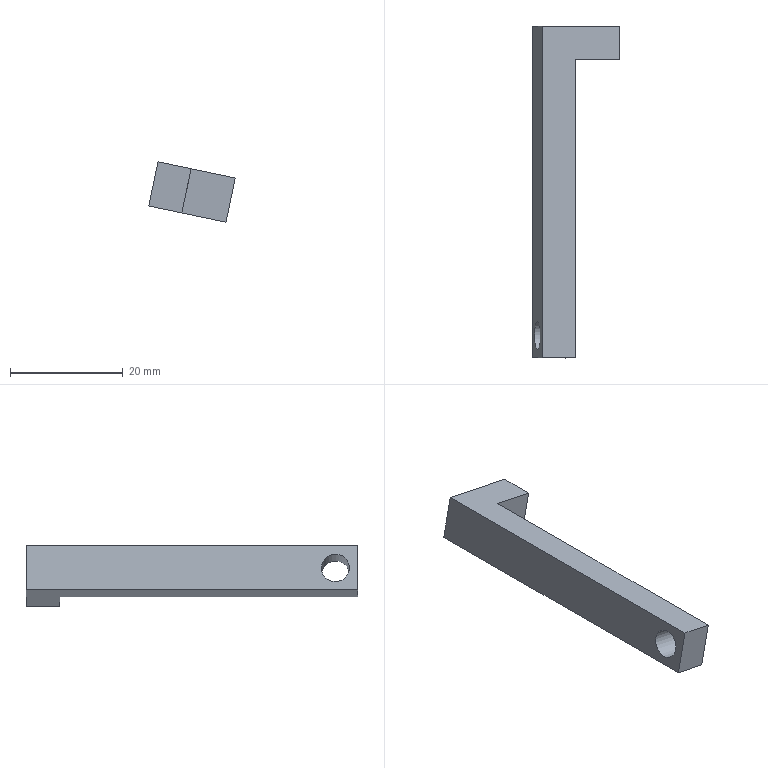Part | STEP file | SN10_006_003_GUIA | 1 solid | 9 faces | box 15.346 x 59 x 10.708 mm | volume 3098 mm3 | plane 8 | cylinder 1 | commonest cylinder face diameters 5 x1
STEP:
#1=CARTESIAN_POINT('',(0.,0.,0.));
#2=DIRECTION('',(0.,0.,1.));
#3=DIRECTION('',(1.,0.,0.));
#4=AXIS2_PLACEMENT_3D('',#1,#2,#3);
#5=CARTESIAN_POINT('',(355.51,-536.049,335.898));
#6=VERTEX_POINT('',#5);
#7=CARTESIAN_POINT('',(355.059,-534.85,333.75));
#8=DIRECTION('',(-0.9786,0.,0.2056));
#9=DIRECTION('',(0.2056,0.,0.9786));
#10=AXIS2_PLACEMENT_3D('',#7,#8,#9);
#11=CIRCLE('',#10,2.5);
#12=CARTESIAN_POINT('',(355.157,-534.85,333.73));
#13=DIRECTION('',(0.9786,0.,-0.2056));
#14=DIRECTION('',(0.1805,-0.4794,0.8588));
#15=AXIS2_PLACEMENT_3D('',#12,#13,#14);
#16=CYLINDRICAL_SURFACE('',#15,2.5);
#17=CARTESIAN_POINT('',(12.066,-0.1));
#18=DIRECTION('',(-1.,0.));
#19=VECTOR('',#18,1.);
#20=LINE('',#17,#19);
#21=(GEOMETRIC_REPRESENTATION_CONTEXT(2)PARAMETRIC_REPRESENTATION_CONTEXT()REPRESENTATION_CONTEXT('',''));
#22=DEFINITIONAL_REPRESENTATION('',(#20),#21);
#23=PCURVE('',#16,#22);
#24=CARTESIAN_POINT('',(355.059,-479.85,333.75));
#25=DIRECTION('',(-0.9786,0.,0.2056));
#26=DIRECTION('',(0.2056,0.,0.9786));
#27=AXIS2_PLACEMENT_3D('',#24,#25,#26);
#28=PLANE('',#27);
#29=CARTESIAN_POINT('',(0.,-55.));
#30=DIRECTION('',(1.,0.));
#31=AXIS2_PLACEMENT_2D('',#29,#30);
#32=CIRCLE('',#31,2.5);
#33=(GEOMETRIC_REPRESENTATION_CONTEXT(2)PARAMETRIC_REPRESENTATION_CONTEXT()REPRESENTATION_CONTEXT('',''));
#34=DEFINITIONAL_REPRESENTATION('',(#32),#33);
#35=PCURVE('',#28,#34);
#36=SURFACE_CURVE('',#11,(#23,#35),.PCURVE_S1.);
#37=EDGE_CURVE('',#6,#6,#36,.T.);
#38=ORIENTED_EDGE('',*,*,#37,.F.);
#39=CARTESIAN_POINT('',(361.382,-536.049,334.664));
#40=VERTEX_POINT('',#39);
#41=CARTESIAN_POINT('',(355.51,-536.049,335.898));
#42=CARTESIAN_POINT('',(361.382,-536.049,334.664));
#43=B_SPLINE_CURVE_WITH_KNOTS('',1,(#41,#42),.UNSPECIFIED.,.F.,.F.,(2,2),(-0.1,5.9),.PIECEWISE_BEZIER_KNOTS.);
#44=CARTESIAN_POINT('',(6.283,0.));
#45=DIRECTION('',(0.,1.));
#46=VECTOR('',#45,1.);
#47=LINE('',#44,#46);
#48=(GEOMETRIC_REPRESENTATION_CONTEXT(2)PARAMETRIC_REPRESENTATION_CONTEXT()REPRESENTATION_CONTEXT('',''));
#49=DEFINITIONAL_REPRESENTATION('',(#47),#48);
#50=PCURVE('',#16,#49);
#51=CARTESIAN_POINT('',(0.,0.));
#52=DIRECTION('',(0.,1.));
#53=VECTOR('',#52,1.);
#54=LINE('',#51,#53);
#55=(GEOMETRIC_REPRESENTATION_CONTEXT(2)PARAMETRIC_REPRESENTATION_CONTEXT()REPRESENTATION_CONTEXT('',''));
#56=DEFINITIONAL_REPRESENTATION('',(#54),#55);
#57=PCURVE('',#16,#56);
#58=SEAM_CURVE('',#43,(#50,#57),.PCURVE_S1.);
#59=EDGE_CURVE('',#6,#40,#58,.T.);
#60=ORIENTED_EDGE('',*,*,#59,.T.);
#61=CARTESIAN_POINT('',(360.931,-534.85,332.517));
#62=DIRECTION('',(0.9786,0.,-0.2056));
#63=DIRECTION('',(0.2056,0.,0.9786));
#64=AXIS2_PLACEMENT_3D('',#61,#62,#63);
#65=CIRCLE('',#64,2.5);
#66=CARTESIAN_POINT('',(-0.5,5.9));
#67=DIRECTION('',(1.,0.));
#68=VECTOR('',#67,1.);
#69=LINE('',#66,#68);
#70=(GEOMETRIC_REPRESENTATION_CONTEXT(2)PARAMETRIC_REPRESENTATION_CONTEXT()REPRESENTATION_CONTEXT('',''));
#71=DEFINITIONAL_REPRESENTATION('',(#69),#70);
#72=PCURVE('',#16,#71);
#73=CARTESIAN_POINT('',(360.931,-538.85,332.517));
#74=DIRECTION('',(0.9786,0.,-0.2056));
#75=DIRECTION('',(-0.2056,0.,-0.9786));
#76=AXIS2_PLACEMENT_3D('',#73,#74,#75);
#77=PLANE('',#76);
#78=CARTESIAN_POINT('',(0.,4.));
#79=DIRECTION('',(-1.,0.));
#80=AXIS2_PLACEMENT_2D('',#78,#79);
#81=CIRCLE('',#80,2.5);
#82=(GEOMETRIC_REPRESENTATION_CONTEXT(2)PARAMETRIC_REPRESENTATION_CONTEXT()REPRESENTATION_CONTEXT('',''));
#83=DEFINITIONAL_REPRESENTATION('',(#81),#82);
#84=PCURVE('',#77,#83);
#85=SURFACE_CURVE('',#65,(#72,#84),.PCURVE_S1.);
#86=EDGE_CURVE('',#40,#40,#85,.T.);
#87=ORIENTED_EDGE('',*,*,#86,.F.);
#88=ORIENTED_EDGE('',*,*,#59,.F.);
#89=EDGE_LOOP('',(#38,#60,#87,#88));
#90=FACE_BOUND('',#89,.F.);
#91=ADVANCED_FACE('',(#90),#16,.F.);
#92=CARTESIAN_POINT('',(354.236,-479.85,329.836));
#93=VERTEX_POINT('',#92);
#94=CARTESIAN_POINT('',(355.882,-479.85,337.665));
#95=VERTEX_POINT('',#94);
#96=CARTESIAN_POINT('',(354.236,-479.85,329.836));
#97=DIRECTION('',(0.2056,0.,0.9786));
#98=VECTOR('',#97,1.);
#99=LINE('',#96,#98);
#100=CARTESIAN_POINT('',(-4.,0.));
#101=DIRECTION('',(1.,0.));
#102=VECTOR('',#101,1.);
#103=LINE('',#100,#102);
#104=(GEOMETRIC_REPRESENTATION_CONTEXT(2)PARAMETRIC_REPRESENTATION_CONTEXT()REPRESENTATION_CONTEXT('',''));
#105=DEFINITIONAL_REPRESENTATION('',(#103),#104);
#106=PCURVE('',#28,#105);
#107=CARTESIAN_POINT('',(368.76,-479.85,330.871));
#108=DIRECTION('',(0.,1.,0.));
#109=DIRECTION('',(0.,0.,1.));
#110=AXIS2_PLACEMENT_3D('',#107,#108,#109);
#111=PLANE('',#110);
#112=CARTESIAN_POINT('',(-1.036,-14.523));
#113=DIRECTION('',(0.9786,0.2056));
#114=VECTOR('',#113,1.);
#115=LINE('',#112,#114);
#116=(GEOMETRIC_REPRESENTATION_CONTEXT(2)PARAMETRIC_REPRESENTATION_CONTEXT()REPRESENTATION_CONTEXT('',''));
#117=DEFINITIONAL_REPRESENTATION('',(#115),#116);
#118=PCURVE('',#111,#117);
#119=SURFACE_CURVE('',#99,(#106,#118),.PCURVE_S1.);
#120=EDGE_CURVE('',#93,#95,#119,.T.);
#121=ORIENTED_EDGE('',*,*,#120,.F.);
#122=CARTESIAN_POINT('',(354.236,-538.85,329.836));
#123=VERTEX_POINT('',#122);
#124=CARTESIAN_POINT('',(354.236,-479.85,329.836));
#125=DIRECTION('',(0.,-1.,0.));
#126=VECTOR('',#125,1.);
#127=LINE('',#124,#126);
#128=CARTESIAN_POINT('',(-4.,0.));
#129=DIRECTION('',(0.,-1.));
#130=VECTOR('',#129,1.);
#131=LINE('',#128,#130);
#132=(GEOMETRIC_REPRESENTATION_CONTEXT(2)PARAMETRIC_REPRESENTATION_CONTEXT()REPRESENTATION_CONTEXT('',''));
#133=DEFINITIONAL_REPRESENTATION('',(#131),#132);
#134=PCURVE('',#28,#133);
#135=CARTESIAN_POINT('',(360.108,-534.85,328.602));
#136=DIRECTION('',(0.2056,0.,0.9786));
#137=DIRECTION('',(0.9786,0.,-0.2056));
#138=AXIS2_PLACEMENT_3D('',#135,#136,#137);
#139=PLANE('',#138);
#140=CARTESIAN_POINT('',(-6.,55.));
#141=DIRECTION('',(0.,-1.));
#142=VECTOR('',#141,1.);
#143=LINE('',#140,#142);
#144=(GEOMETRIC_REPRESENTATION_CONTEXT(2)PARAMETRIC_REPRESENTATION_CONTEXT()REPRESENTATION_CONTEXT('',''));
#145=DEFINITIONAL_REPRESENTATION('',(#143),#144);
#146=PCURVE('',#139,#145);
#147=SURFACE_CURVE('',#127,(#134,#146),.PCURVE_S1.);
#148=EDGE_CURVE('',#93,#123,#147,.T.);
#149=ORIENTED_EDGE('',*,*,#148,.T.);
#150=CARTESIAN_POINT('',(355.882,-538.85,337.665));
#151=VERTEX_POINT('',#150);
#152=CARTESIAN_POINT('',(354.236,-538.85,329.836));
#153=DIRECTION('',(0.2056,0.,0.9786));
#154=VECTOR('',#153,1.);
#155=LINE('',#152,#154);
#156=CARTESIAN_POINT('',(-4.,-59.));
#157=DIRECTION('',(1.,0.));
#158=VECTOR('',#157,1.);
#159=LINE('',#156,#158);
#160=(GEOMETRIC_REPRESENTATION_CONTEXT(2)PARAMETRIC_REPRESENTATION_CONTEXT()REPRESENTATION_CONTEXT('',''));
#161=DEFINITIONAL_REPRESENTATION('',(#159),#160);
#162=PCURVE('',#28,#161);
#163=CARTESIAN_POINT('',(355.059,-538.85,333.75));
#164=DIRECTION('',(0.,-1.,0.));
#165=DIRECTION('',(0.,0.,-1.));
#166=AXIS2_PLACEMENT_3D('',#163,#164,#165);
#167=PLANE('',#166);
#168=CARTESIAN_POINT('',(3.915,-0.8226));
#169=DIRECTION('',(-0.9786,0.2056));
#170=VECTOR('',#169,1.);
#171=LINE('',#168,#170);
#172=(GEOMETRIC_REPRESENTATION_CONTEXT(2)PARAMETRIC_REPRESENTATION_CONTEXT()REPRESENTATION_CONTEXT('',''));
#173=DEFINITIONAL_REPRESENTATION('',(#171),#172);
#174=PCURVE('',#167,#173);
#175=SURFACE_CURVE('',#155,(#162,#174),.PCURVE_S1.);
#176=EDGE_CURVE('',#123,#151,#175,.T.);
#177=ORIENTED_EDGE('',*,*,#176,.T.);
#178=CARTESIAN_POINT('',(355.882,-479.85,337.665));
#179=DIRECTION('',(0.,-1.,0.));
#180=VECTOR('',#179,1.);
#181=LINE('',#178,#180);
#182=CARTESIAN_POINT('',(4.,0.));
#183=DIRECTION('',(0.,-1.));
#184=VECTOR('',#183,1.);
#185=LINE('',#182,#184);
#186=(GEOMETRIC_REPRESENTATION_CONTEXT(2)PARAMETRIC_REPRESENTATION_CONTEXT()REPRESENTATION_CONTEXT('',''));
#187=DEFINITIONAL_REPRESENTATION('',(#185),#186);
#188=PCURVE('',#28,#187);
#189=CARTESIAN_POINT('',(361.753,-534.85,336.431));
#190=DIRECTION('',(0.2056,0.,0.9786));
#191=DIRECTION('',(0.9786,0.,-0.2056));
#192=AXIS2_PLACEMENT_3D('',#189,#190,#191);
#193=PLANE('',#192);
#194=CARTESIAN_POINT('',(-6.,55.));
#195=DIRECTION('',(0.,-1.));
#196=VECTOR('',#195,1.);
#197=LINE('',#194,#196);
#198=(GEOMETRIC_REPRESENTATION_CONTEXT(2)PARAMETRIC_REPRESENTATION_CONTEXT()REPRESENTATION_CONTEXT('',''));
#199=DEFINITIONAL_REPRESENTATION('',(#197),#198);
#200=PCURVE('',#193,#199);
#201=SURFACE_CURVE('',#181,(#188,#200),.PCURVE_S1.);
#202=EDGE_CURVE('',#95,#151,#201,.T.);
#203=ORIENTED_EDGE('',*,*,#202,.F.);
#204=EDGE_LOOP('',(#121,#149,#177,#203));
#205=FACE_BOUND('',#204,.T.);
#206=ORIENTED_EDGE('',*,*,#37,.F.);
#207=EDGE_LOOP('',(#206));
#208=FACE_BOUND('',#207,.T.);
#209=ADVANCED_FACE('',(#205,#208),#28,.T.);
#210=CARTESIAN_POINT('',(360.108,-538.85,328.602));
#211=VERTEX_POINT('',#210);
#212=CARTESIAN_POINT('',(361.753,-538.85,336.431));
#213=VERTEX_POINT('',#212);
#214=CARTESIAN_POINT('',(360.108,-538.85,328.602));
#215=DIRECTION('',(0.2056,0.,0.9786));
#216=VECTOR('',#215,1.);
#217=LINE('',#214,#216);
#218=CARTESIAN_POINT('',(4.,0.));
#219=DIRECTION('',(-1.,0.));
#220=VECTOR('',#219,1.);
#221=LINE('',#218,#220);
#222=(GEOMETRIC_REPRESENTATION_CONTEXT(2)PARAMETRIC_REPRESENTATION_CONTEXT()REPRESENTATION_CONTEXT('',''));
#223=DEFINITIONAL_REPRESENTATION('',(#221),#222);
#224=PCURVE('',#77,#223);
#225=CARTESIAN_POINT('',(5.148,5.049));
#226=DIRECTION('',(-0.9786,0.2056));
#227=VECTOR('',#226,1.);
#228=LINE('',#225,#227);
#229=(GEOMETRIC_REPRESENTATION_CONTEXT(2)PARAMETRIC_REPRESENTATION_CONTEXT()REPRESENTATION_CONTEXT('',''));
#230=DEFINITIONAL_REPRESENTATION('',(#228),#229);
#231=PCURVE('',#167,#230);
#232=SURFACE_CURVE('',#217,(#224,#231),.PCURVE_S1.);
#233=EDGE_CURVE('',#211,#213,#232,.T.);
#234=ORIENTED_EDGE('',*,*,#233,.F.);
#235=CARTESIAN_POINT('',(360.108,-485.85,328.602));
#236=VERTEX_POINT('',#235);
#237=CARTESIAN_POINT('',(360.108,-538.85,328.602));
#238=DIRECTION('',(0.,1.,0.));
#239=VECTOR('',#238,1.);
#240=LINE('',#237,#239);
#241=CARTESIAN_POINT('',(4.,0.));
#242=DIRECTION('',(0.,1.));
#243=VECTOR('',#242,1.);
#244=LINE('',#241,#243);
#245=(GEOMETRIC_REPRESENTATION_CONTEXT(2)PARAMETRIC_REPRESENTATION_CONTEXT()REPRESENTATION_CONTEXT('',''));
#246=DEFINITIONAL_REPRESENTATION('',(#244),#245);
#247=PCURVE('',#77,#246);
#248=CARTESIAN_POINT('',(0.,-4.));
#249=DIRECTION('',(0.,1.));
#250=VECTOR('',#249,1.);
#251=LINE('',#248,#250);
#252=(GEOMETRIC_REPRESENTATION_CONTEXT(2)PARAMETRIC_REPRESENTATION_CONTEXT()REPRESENTATION_CONTEXT('',''));
#253=DEFINITIONAL_REPRESENTATION('',(#251),#252);
#254=PCURVE('',#139,#253);
#255=SURFACE_CURVE('',#240,(#247,#254),.PCURVE_S1.);
#256=EDGE_CURVE('',#211,#236,#255,.T.);
#257=ORIENTED_EDGE('',*,*,#256,.T.);
#258=CARTESIAN_POINT('',(361.753,-485.85,336.431));
#259=VERTEX_POINT('',#258);
#260=CARTESIAN_POINT('',(360.108,-485.85,328.602));
#261=DIRECTION('',(0.2056,0.,0.9786));
#262=VECTOR('',#261,1.);
#263=LINE('',#260,#262);
#264=CARTESIAN_POINT('',(4.,53.));
#265=DIRECTION('',(-1.,0.));
#266=VECTOR('',#265,1.);
#267=LINE('',#264,#266);
#268=(GEOMETRIC_REPRESENTATION_CONTEXT(2)PARAMETRIC_REPRESENTATION_CONTEXT()REPRESENTATION_CONTEXT('',''));
#269=DEFINITIONAL_REPRESENTATION('',(#267),#268);
#270=PCURVE('',#77,#269);
#271=CARTESIAN_POINT('',(360.931,-485.85,332.517));
#272=DIRECTION('',(0.,-1.,0.));
#273=DIRECTION('',(0.,0.,-1.));
#274=AXIS2_PLACEMENT_3D('',#271,#272,#273);
#275=PLANE('',#274);
#276=CARTESIAN_POINT('',(3.915,-0.8226));
#277=DIRECTION('',(-0.9786,0.2056));
#278=VECTOR('',#277,1.);
#279=LINE('',#276,#278);
#280=(GEOMETRIC_REPRESENTATION_CONTEXT(2)PARAMETRIC_REPRESENTATION_CONTEXT()REPRESENTATION_CONTEXT('',''));
#281=DEFINITIONAL_REPRESENTATION('',(#279),#280);
#282=PCURVE('',#275,#281);
#283=SURFACE_CURVE('',#263,(#270,#282),.PCURVE_S1.);
#284=EDGE_CURVE('',#236,#259,#283,.T.);
#285=ORIENTED_EDGE('',*,*,#284,.T.);
#286=CARTESIAN_POINT('',(361.753,-538.85,336.431));
#287=DIRECTION('',(0.,1.,0.));
#288=VECTOR('',#287,1.);
#289=LINE('',#286,#288);
#290=CARTESIAN_POINT('',(-4.,0.));
#291=DIRECTION('',(0.,1.));
#292=VECTOR('',#291,1.);
#293=LINE('',#290,#292);
#294=(GEOMETRIC_REPRESENTATION_CONTEXT(2)PARAMETRIC_REPRESENTATION_CONTEXT()REPRESENTATION_CONTEXT('',''));
#295=DEFINITIONAL_REPRESENTATION('',(#293),#294);
#296=PCURVE('',#77,#295);
#297=CARTESIAN_POINT('',(0.,-4.));
#298=DIRECTION('',(0.,1.));
#299=VECTOR('',#298,1.);
#300=LINE('',#297,#299);
#301=(GEOMETRIC_REPRESENTATION_CONTEXT(2)PARAMETRIC_REPRESENTATION_CONTEXT()REPRESENTATION_CONTEXT('',''));
#302=DEFINITIONAL_REPRESENTATION('',(#300),#301);
#303=PCURVE('',#193,#302);
#304=SURFACE_CURVE('',#289,(#296,#303),.PCURVE_S1.);
#305=EDGE_CURVE('',#213,#259,#304,.T.);
#306=ORIENTED_EDGE('',*,*,#305,.F.);
#307=EDGE_LOOP('',(#234,#257,#285,#306));
#308=FACE_BOUND('',#307,.T.);
#309=ORIENTED_EDGE('',*,*,#86,.F.);
#310=EDGE_LOOP('',(#309));
#311=FACE_BOUND('',#310,.T.);
#312=ADVANCED_FACE('',(#308,#311),#77,.T.);
#313=CARTESIAN_POINT('',(354.236,-538.85,329.836));
#314=DIRECTION('',(0.9786,0.,-0.2056));
#315=VECTOR('',#314,1.);
#316=LINE('',#313,#315);
#317=CARTESIAN_POINT('',(-6.,-4.));
#318=DIRECTION('',(1.,0.));
#319=VECTOR('',#318,1.);
#320=LINE('',#317,#319);
#321=(GEOMETRIC_REPRESENTATION_CONTEXT(2)PARAMETRIC_REPRESENTATION_CONTEXT()REPRESENTATION_CONTEXT('',''));
#322=DEFINITIONAL_REPRESENTATION('',(#320),#321);
#323=PCURVE('',#139,#322);
#324=CARTESIAN_POINT('',(3.915,-0.8226));
#325=DIRECTION('',(0.2056,0.9786));
#326=VECTOR('',#325,1.);
#327=LINE('',#324,#326);
#328=(GEOMETRIC_REPRESENTATION_CONTEXT(2)PARAMETRIC_REPRESENTATION_CONTEXT()REPRESENTATION_CONTEXT('',''));
#329=DEFINITIONAL_REPRESENTATION('',(#327),#328);
#330=PCURVE('',#167,#329);
#331=SURFACE_CURVE('',#316,(#323,#330),.PCURVE_S1.);
#332=EDGE_CURVE('',#123,#211,#331,.T.);
#333=ORIENTED_EDGE('',*,*,#332,.F.);
#334=ORIENTED_EDGE('',*,*,#148,.F.);
#335=CARTESIAN_POINT('',(367.937,-479.85,326.957));
#336=VERTEX_POINT('',#335);
#337=CARTESIAN_POINT('',(367.937,-479.85,326.957));
#338=DIRECTION('',(-0.9786,0.,0.2056));
#339=VECTOR('',#338,1.);
#340=LINE('',#337,#339);
#341=CARTESIAN_POINT('',(8.,55.));
#342=DIRECTION('',(-1.,0.));
#343=VECTOR('',#342,1.);
#344=LINE('',#341,#343);
#345=(GEOMETRIC_REPRESENTATION_CONTEXT(2)PARAMETRIC_REPRESENTATION_CONTEXT()REPRESENTATION_CONTEXT('',''));
#346=DEFINITIONAL_REPRESENTATION('',(#344),#345);
#347=PCURVE('',#139,#346);
#348=CARTESIAN_POINT('',(-3.915,-0.8226));
#349=DIRECTION('',(0.2056,-0.9786));
#350=VECTOR('',#349,1.);
#351=LINE('',#348,#350);
#352=(GEOMETRIC_REPRESENTATION_CONTEXT(2)PARAMETRIC_REPRESENTATION_CONTEXT()REPRESENTATION_CONTEXT('',''));
#353=DEFINITIONAL_REPRESENTATION('',(#351),#352);
#354=PCURVE('',#111,#353);
#355=SURFACE_CURVE('',#340,(#347,#354),.PCURVE_S1.);
#356=EDGE_CURVE('',#336,#93,#355,.T.);
#357=ORIENTED_EDGE('',*,*,#356,.F.);
#358=CARTESIAN_POINT('',(367.937,-485.85,326.957));
#359=VERTEX_POINT('',#358);
#360=CARTESIAN_POINT('',(367.937,-485.85,326.957));
#361=DIRECTION('',(0.,1.,0.));
#362=VECTOR('',#361,1.);
#363=LINE('',#360,#362);
#364=CARTESIAN_POINT('',(8.,49.));
#365=DIRECTION('',(0.,1.));
#366=VECTOR('',#365,1.);
#367=LINE('',#364,#366);
#368=(GEOMETRIC_REPRESENTATION_CONTEXT(2)PARAMETRIC_REPRESENTATION_CONTEXT()REPRESENTATION_CONTEXT('',''));
#369=DEFINITIONAL_REPRESENTATION('',(#367),#368);
#370=PCURVE('',#139,#369);
#371=CARTESIAN_POINT('',(368.76,-485.85,330.871));
#372=DIRECTION('',(0.9786,0.,-0.2056));
#373=DIRECTION('',(-0.2056,0.,-0.9786));
#374=AXIS2_PLACEMENT_3D('',#371,#372,#373);
#375=PLANE('',#374);
#376=CARTESIAN_POINT('',(4.,0.));
#377=DIRECTION('',(0.,1.));
#378=VECTOR('',#377,1.);
#379=LINE('',#376,#378);
#380=(GEOMETRIC_REPRESENTATION_CONTEXT(2)PARAMETRIC_REPRESENTATION_CONTEXT()REPRESENTATION_CONTEXT('',''));
#381=DEFINITIONAL_REPRESENTATION('',(#379),#380);
#382=PCURVE('',#375,#381);
#383=SURFACE_CURVE('',#363,(#370,#382),.PCURVE_S1.);
#384=EDGE_CURVE('',#359,#336,#383,.T.);
#385=ORIENTED_EDGE('',*,*,#384,.F.);
#386=CARTESIAN_POINT('',(360.108,-485.85,328.602));
#387=DIRECTION('',(0.9786,0.,-0.2056));
#388=VECTOR('',#387,1.);
#389=LINE('',#386,#388);
#390=CARTESIAN_POINT('',(0.,49.));
#391=DIRECTION('',(1.,0.));
#392=VECTOR('',#391,1.);
#393=LINE('',#390,#392);
#394=(GEOMETRIC_REPRESENTATION_CONTEXT(2)PARAMETRIC_REPRESENTATION_CONTEXT()REPRESENTATION_CONTEXT('',''));
#395=DEFINITIONAL_REPRESENTATION('',(#393),#394);
#396=PCURVE('',#139,#395);
#397=CARTESIAN_POINT('',(3.915,-0.8226));
#398=DIRECTION('',(0.2056,0.9786));
#399=VECTOR('',#398,1.);
#400=LINE('',#397,#399);
#401=(GEOMETRIC_REPRESENTATION_CONTEXT(2)PARAMETRIC_REPRESENTATION_CONTEXT()REPRESENTATION_CONTEXT('',''));
#402=DEFINITIONAL_REPRESENTATION('',(#400),#401);
#403=PCURVE('',#275,#402);
#404=SURFACE_CURVE('',#389,(#396,#403),.PCURVE_S1.);
#405=EDGE_CURVE('',#236,#359,#404,.T.);
#406=ORIENTED_EDGE('',*,*,#405,.F.);
#407=ORIENTED_EDGE('',*,*,#256,.F.);
#408=EDGE_LOOP('',(#333,#334,#357,#385,#406,#407));
#409=FACE_BOUND('',#408,.T.);
#410=ADVANCED_FACE('',(#409),#139,.F.);
#411=ORIENTED_EDGE('',*,*,#176,.F.);
#412=ORIENTED_EDGE('',*,*,#332,.T.);
#413=ORIENTED_EDGE('',*,*,#233,.T.);
#414=CARTESIAN_POINT('',(355.882,-538.85,337.665));
#415=DIRECTION('',(0.9786,0.,-0.2056));
#416=VECTOR('',#415,1.);
#417=LINE('',#414,#416);
#418=CARTESIAN_POINT('',(-3.915,0.8226));
#419=DIRECTION('',(0.2056,0.9786));
#420=VECTOR('',#419,1.);
#421=LINE('',#418,#420);
#422=(GEOMETRIC_REPRESENTATION_CONTEXT(2)PARAMETRIC_REPRESENTATION_CONTEXT()REPRESENTATION_CONTEXT('',''));
#423=DEFINITIONAL_REPRESENTATION('',(#421),#422);
#424=PCURVE('',#167,#423);
#425=CARTESIAN_POINT('',(-6.,-4.));
#426=DIRECTION('',(1.,0.));
#427=VECTOR('',#426,1.);
#428=LINE('',#425,#427);
#429=(GEOMETRIC_REPRESENTATION_CONTEXT(2)PARAMETRIC_REPRESENTATION_CONTEXT()REPRESENTATION_CONTEXT('',''));
#430=DEFINITIONAL_REPRESENTATION('',(#428),#429);
#431=PCURVE('',#193,#430);
#432=SURFACE_CURVE('',#417,(#424,#431),.PCURVE_S1.);
#433=EDGE_CURVE('',#151,#213,#432,.T.);
#434=ORIENTED_EDGE('',*,*,#433,.F.);
#435=EDGE_LOOP('',(#411,#412,#413,#434));
#436=FACE_BOUND('',#435,.T.);
#437=ADVANCED_FACE('',(#436),#167,.T.);
#438=ORIENTED_EDGE('',*,*,#284,.F.);
#439=ORIENTED_EDGE('',*,*,#405,.T.);
#440=CARTESIAN_POINT('',(369.582,-485.85,334.786));
#441=VERTEX_POINT('',#440);
#442=CARTESIAN_POINT('',(367.937,-485.85,326.957));
#443=DIRECTION('',(0.2056,0.,0.9786));
#444=VECTOR('',#443,1.);
#445=LINE('',#442,#444);
#446=CARTESIAN_POINT('',(5.56,7.006));
#447=DIRECTION('',(-0.9786,0.2056));
#448=VECTOR('',#447,1.);
#449=LINE('',#446,#448);
#450=(GEOMETRIC_REPRESENTATION_CONTEXT(2)PARAMETRIC_REPRESENTATION_CONTEXT()REPRESENTATION_CONTEXT('',''));
#451=DEFINITIONAL_REPRESENTATION('',(#449),#450);
#452=PCURVE('',#275,#451);
#453=CARTESIAN_POINT('',(4.,0.));
#454=DIRECTION('',(-1.,0.));
#455=VECTOR('',#454,1.);
#456=LINE('',#453,#455);
#457=(GEOMETRIC_REPRESENTATION_CONTEXT(2)PARAMETRIC_REPRESENTATION_CONTEXT()REPRESENTATION_CONTEXT('',''));
#458=DEFINITIONAL_REPRESENTATION('',(#456),#457);
#459=PCURVE('',#375,#458);
#460=SURFACE_CURVE('',#445,(#452,#459),.PCURVE_S1.);
#461=EDGE_CURVE('',#359,#441,#460,.T.);
#462=ORIENTED_EDGE('',*,*,#461,.T.);
#463=CARTESIAN_POINT('',(361.753,-485.85,336.431));
#464=DIRECTION('',(0.9786,0.,-0.2056));
#465=VECTOR('',#464,1.);
#466=LINE('',#463,#465);
#467=CARTESIAN_POINT('',(-3.915,0.8226));
#468=DIRECTION('',(0.2056,0.9786));
#469=VECTOR('',#468,1.);
#470=LINE('',#467,#469);
#471=(GEOMETRIC_REPRESENTATION_CONTEXT(2)PARAMETRIC_REPRESENTATION_CONTEXT()REPRESENTATION_CONTEXT('',''));
#472=DEFINITIONAL_REPRESENTATION('',(#470),#471);
#473=PCURVE('',#275,#472);
#474=CARTESIAN_POINT('',(0.,49.));
#475=DIRECTION('',(1.,0.));
#476=VECTOR('',#475,1.);
#477=LINE('',#474,#476);
#478=(GEOMETRIC_REPRESENTATION_CONTEXT(2)PARAMETRIC_REPRESENTATION_CONTEXT()REPRESENTATION_CONTEXT('',''));
#479=DEFINITIONAL_REPRESENTATION('',(#477),#478);
#480=PCURVE('',#193,#479);
#481=SURFACE_CURVE('',#466,(#473,#480),.PCURVE_S1.);
#482=EDGE_CURVE('',#259,#441,#481,.T.);
#483=ORIENTED_EDGE('',*,*,#482,.F.);
#484=EDGE_LOOP('',(#438,#439,#462,#483));
#485=FACE_BOUND('',#484,.T.);
#486=ADVANCED_FACE('',(#485),#275,.T.);
#487=ORIENTED_EDGE('',*,*,#461,.F.);
#488=ORIENTED_EDGE('',*,*,#384,.T.);
#489=CARTESIAN_POINT('',(369.582,-479.85,334.786));
#490=VERTEX_POINT('',#489);
#491=CARTESIAN_POINT('',(367.937,-479.85,326.957));
#492=DIRECTION('',(0.2056,0.,0.9786));
#493=VECTOR('',#492,1.);
#494=LINE('',#491,#493);
#495=CARTESIAN_POINT('',(4.,6.));
#496=DIRECTION('',(-1.,0.));
#497=VECTOR('',#496,1.);
#498=LINE('',#495,#497);
#499=(GEOMETRIC_REPRESENTATION_CONTEXT(2)PARAMETRIC_REPRESENTATION_CONTEXT()REPRESENTATION_CONTEXT('',''));
#500=DEFINITIONAL_REPRESENTATION('',(#498),#499);
#501=PCURVE('',#375,#500);
#502=CARTESIAN_POINT('',(-3.915,-0.8226));
#503=DIRECTION('',(0.9786,0.2056));
#504=VECTOR('',#503,1.);
#505=LINE('',#502,#504);
#506=(GEOMETRIC_REPRESENTATION_CONTEXT(2)PARAMETRIC_REPRESENTATION_CONTEXT()REPRESENTATION_CONTEXT('',''));
#507=DEFINITIONAL_REPRESENTATION('',(#505),#506);
#508=PCURVE('',#111,#507);
#509=SURFACE_CURVE('',#494,(#501,#508),.PCURVE_S1.);
#510=EDGE_CURVE('',#336,#490,#509,.T.);
#511=ORIENTED_EDGE('',*,*,#510,.T.);
#512=CARTESIAN_POINT('',(369.582,-485.85,334.786));
#513=DIRECTION('',(0.,1.,0.));
#514=VECTOR('',#513,1.);
#515=LINE('',#512,#514);
#516=CARTESIAN_POINT('',(-4.,0.));
#517=DIRECTION('',(0.,1.));
#518=VECTOR('',#517,1.);
#519=LINE('',#516,#518);
#520=(GEOMETRIC_REPRESENTATION_CONTEXT(2)PARAMETRIC_REPRESENTATION_CONTEXT()REPRESENTATION_CONTEXT('',''));
#521=DEFINITIONAL_REPRESENTATION('',(#519),#520);
#522=PCURVE('',#375,#521);
#523=CARTESIAN_POINT('',(8.,49.));
#524=DIRECTION('',(0.,1.));
#525=VECTOR('',#524,1.);
#526=LINE('',#523,#525);
#527=(GEOMETRIC_REPRESENTATION_CONTEXT(2)PARAMETRIC_REPRESENTATION_CONTEXT()REPRESENTATION_CONTEXT('',''));
#528=DEFINITIONAL_REPRESENTATION('',(#526),#527);
#529=PCURVE('',#193,#528);
#530=SURFACE_CURVE('',#515,(#522,#529),.PCURVE_S1.);
#531=EDGE_CURVE('',#441,#490,#530,.T.);
#532=ORIENTED_EDGE('',*,*,#531,.F.);
#533=EDGE_LOOP('',(#487,#488,#511,#532));
#534=FACE_BOUND('',#533,.T.);
#535=ADVANCED_FACE('',(#534),#375,.T.);
#536=ORIENTED_EDGE('',*,*,#305,.T.);
#537=ORIENTED_EDGE('',*,*,#482,.T.);
#538=ORIENTED_EDGE('',*,*,#531,.T.);
#539=CARTESIAN_POINT('',(369.582,-479.85,334.786));
#540=DIRECTION('',(-0.9786,0.,0.2056));
#541=VECTOR('',#540,1.);
#542=LINE('',#539,#541);
#543=CARTESIAN_POINT('',(8.,55.));
#544=DIRECTION('',(-1.,0.));
#545=VECTOR('',#544,1.);
#546=LINE('',#543,#545);
#547=(GEOMETRIC_REPRESENTATION_CONTEXT(2)PARAMETRIC_REPRESENTATION_CONTEXT()REPRESENTATION_CONTEXT('',''));
#548=DEFINITIONAL_REPRESENTATION('',(#546),#547);
#549=PCURVE('',#193,#548);
#550=CARTESIAN_POINT('',(3.915,0.8226));
#551=DIRECTION('',(0.2056,-0.9786));
#552=VECTOR('',#551,1.);
#553=LINE('',#550,#552);
#554=(GEOMETRIC_REPRESENTATION_CONTEXT(2)PARAMETRIC_REPRESENTATION_CONTEXT()REPRESENTATION_CONTEXT('',''));
#555=DEFINITIONAL_REPRESENTATION('',(#553),#554);
#556=PCURVE('',#111,#555);
#557=SURFACE_CURVE('',#542,(#549,#556),.PCURVE_S1.);
#558=EDGE_CURVE('',#490,#95,#557,.T.);
#559=ORIENTED_EDGE('',*,*,#558,.T.);
#560=ORIENTED_EDGE('',*,*,#202,.T.);
#561=ORIENTED_EDGE('',*,*,#433,.T.);
#562=EDGE_LOOP('',(#536,#537,#538,#559,#560,#561));
#563=FACE_BOUND('',#562,.T.);
#564=ADVANCED_FACE('',(#563),#193,.T.);
#565=ORIENTED_EDGE('',*,*,#510,.F.);
#566=ORIENTED_EDGE('',*,*,#356,.T.);
#567=ORIENTED_EDGE('',*,*,#120,.T.);
#568=ORIENTED_EDGE('',*,*,#558,.F.);
#569=EDGE_LOOP('',(#565,#566,#567,#568));
#570=FACE_BOUND('',#569,.T.);
#571=ADVANCED_FACE('',(#570),#111,.T.);
#572=CLOSED_SHELL('',(#91,#209,#312,#410,#437,#486,#535,#564,#571));
#573=MANIFOLD_SOLID_BREP('',#572);
#574=(LENGTH_UNIT()NAMED_UNIT(*)SI_UNIT(.MILLI.,.METRE.));
#575=UNCERTAINTY_MEASURE_WITH_UNIT(LENGTH_MEASURE(0.000001),#574,'','');
#576=(NAMED_UNIT(*)PLANE_ANGLE_UNIT()SI_UNIT($,.RADIAN.));
#577=(NAMED_UNIT(*)SI_UNIT($,.STERADIAN.)SOLID_ANGLE_UNIT());
#578=(GEOMETRIC_REPRESENTATION_CONTEXT(3)GLOBAL_UNCERTAINTY_ASSIGNED_CONTEXT((#575))GLOBAL_UNIT_ASSIGNED_CONTEXT((#574,#576,#577))REPRESENTATION_CONTEXT('',''));
#579=ADVANCED_BREP_SHAPE_REPRESENTATION('',(#4,#573),#578);